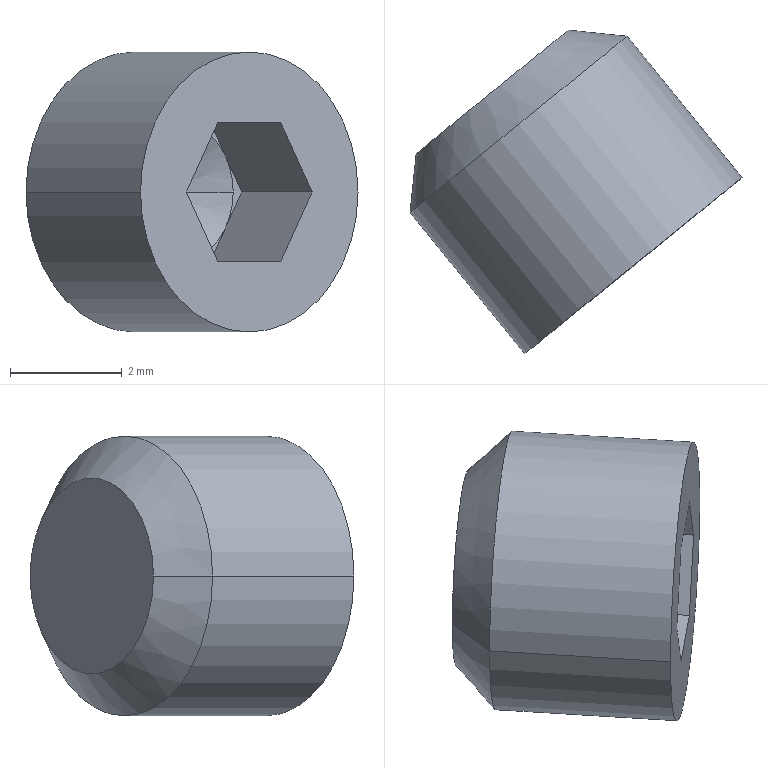Part | SolidWorks | features BaseBody 1 | 1 solid | 20 faces | box 5.931 x 5.783 x 5 mm | volume 62.558 mm3 | plane 14 | cone 4 | cylinder 2 | commonest cylinder face diameters 5 x2
STEP:
#1=CARTESIAN_POINT('',(-125.113,1721.989,-1202.43));
#2=VERTEX_POINT('',#1);
#3=CARTESIAN_POINT('',(-128.998,1718.841,-1202.43));
#4=VERTEX_POINT('',#3);
#5=CARTESIAN_POINT('',(-127.056,1720.415,-1202.43));
#6=DIRECTION('',(0.6296,-0.7769,0.));
#7=DIRECTION('',(0.7769,0.6296,0.));
#8=AXIS2_PLACEMENT_3D('',#5,#6,#7);
#9=CIRCLE('',#8,2.5);
#10=EDGE_CURVE('',#2,#4,#9,.T.);
#11=ORIENTED_EDGE('',*,*,#10,.T.);
#12=CARTESIAN_POINT('',(-126.952,1716.316,-1202.43));
#13=VERTEX_POINT('',#12);
#14=CARTESIAN_POINT('',(-126.952,1716.316,-1202.43));
#15=DIRECTION('',(0.6296,-0.7769,0.));
#16=VECTOR('',#15,1000.);
#17=LINE('',#14,#16);
#18=EDGE_CURVE('',#4,#13,#17,.T.);
#19=ORIENTED_EDGE('',*,*,#18,.T.);
#20=CARTESIAN_POINT('',(-123.067,1719.464,-1202.43));
#21=VERTEX_POINT('',#20);
#22=CARTESIAN_POINT('',(-125.01,1717.89,-1202.43));
#23=DIRECTION('',(-0.6296,0.7769,0.));
#24=DIRECTION('',(0.7769,0.6296,0.));
#25=AXIS2_PLACEMENT_3D('',#22,#23,#24);
#26=CIRCLE('',#25,2.5);
#27=EDGE_CURVE('',#13,#21,#26,.T.);
#28=ORIENTED_EDGE('',*,*,#27,.T.);
#29=CARTESIAN_POINT('',(-123.067,1719.464,-1202.43));
#30=DIRECTION('',(0.6296,-0.7769,0.));
#31=VECTOR('',#30,1000.);
#32=LINE('',#29,#31);
#33=EDGE_CURVE('',#2,#21,#32,.T.);
#34=ORIENTED_EDGE('',*,*,#33,.F.);
#35=EDGE_LOOP('',(#11,#19,#28,#34));
#36=FACE_OUTER_BOUND('',#35,.T.);
#37=CARTESIAN_POINT('',(-125.01,1717.89,-1202.43));
#38=DIRECTION('',(0.6296,-0.7769,0.));
#39=DIRECTION('',(0.7769,0.6296,0.));
#40=AXIS2_PLACEMENT_3D('',#37,#38,#39);
#41=CYLINDRICAL_SURFACE('',#40,2.5);
#42=ADVANCED_FACE('',(#36),#41,.T.);
#43=CARTESIAN_POINT('',(-126.168,1722.1,-1202.43));
#44=VERTEX_POINT('',#43);
#45=CARTESIAN_POINT('',(-128.888,1719.896,-1202.43));
#46=VERTEX_POINT('',#45);
#47=CARTESIAN_POINT('',(-127.528,1720.998,-1202.43));
#48=DIRECTION('',(0.6296,-0.7769,0.));
#49=DIRECTION('',(0.7769,0.6296,0.));
#50=AXIS2_PLACEMENT_3D('',#47,#48,#49);
#51=CIRCLE('',#50,1.75);
#52=EDGE_CURVE('',#44,#46,#51,.T.);
#53=ORIENTED_EDGE('',*,*,#52,.T.);
#54=CARTESIAN_POINT('',(-128.998,1718.841,-1202.43));
#55=DIRECTION('',(-0.1042,-0.9946,0.));
#56=VECTOR('',#55,1000.);
#57=LINE('',#54,#56);
#58=EDGE_CURVE('',#46,#4,#57,.T.);
#59=ORIENTED_EDGE('',*,*,#58,.T.);
#60=ORIENTED_EDGE('',*,*,#10,.F.);
#61=CARTESIAN_POINT('',(-125.113,1721.989,-1202.43));
#62=DIRECTION('',(0.9946,-0.1042,0.));
#63=VECTOR('',#62,1000.);
#64=LINE('',#61,#63);
#65=EDGE_CURVE('',#44,#2,#64,.T.);
#66=ORIENTED_EDGE('',*,*,#65,.F.);
#67=EDGE_LOOP('',(#53,#59,#60,#66));
#68=FACE_OUTER_BOUND('',#67,.T.);
#69=CARTESIAN_POINT('',(-127.056,1720.415,-1202.43));
#70=DIRECTION('',(0.6296,-0.7769,0.));
#71=DIRECTION('',(0.7769,0.6296,0.));
#72=AXIS2_PLACEMENT_3D('',#69,#70,#71);
#73=CONICAL_SURFACE('',#72,2.5,0.7854);
#74=ADVANCED_FACE('',(#68),#73,.T.);
#75=CARTESIAN_POINT('',(-126.723,1720.005,-1202.43));
#76=VERTEX_POINT('',#75);
#77=CARTESIAN_POINT('',(-125.298,1720.231,-1202.43));
#78=VERTEX_POINT('',#77);
#79=CARTESIAN_POINT('',(-125.298,1720.231,-1202.43));
#80=DIRECTION('',(0.9876,0.1568,0.));
#81=VECTOR('',#80,1000.);
#82=LINE('',#79,#81);
#83=EDGE_CURVE('',#76,#78,#82,.T.);
#84=ORIENTED_EDGE('',*,*,#83,.F.);
#85=CARTESIAN_POINT('',(-127.24,1718.657,-1202.43));
#86=VERTEX_POINT('',#85);
#87=CARTESIAN_POINT('',(-127.24,1718.657,-1202.43));
#88=DIRECTION('',(-0.358,-0.9337,0.));
#89=VECTOR('',#88,1000.);
#90=LINE('',#87,#89);
#91=EDGE_CURVE('',#76,#86,#90,.T.);
#92=ORIENTED_EDGE('',*,*,#91,.T.);
#93=CARTESIAN_POINT('',(-127.11,1718.762,-1203.055));
#94=VERTEX_POINT('',#93);
#95=CARTESIAN_POINT('',(-126.269,1719.444,-1202.43));
#96=DIRECTION('',(-0.6296,0.7769,0.));
#97=DIRECTION('',(0.7769,0.6296,0.));
#98=AXIS2_PLACEMENT_3D('',#95,#96,#97);
#99=CIRCLE('',#98,1.25);
#100=EDGE_CURVE('',#94,#86,#99,.T.);
#101=ORIENTED_EDGE('',*,*,#100,.F.);
#102=CARTESIAN_POINT('',(-126.269,1719.444,-1203.68));
#103=VERTEX_POINT('',#102);
#104=CARTESIAN_POINT('',(-126.269,1719.444,-1202.43));
#105=DIRECTION('',(-0.6296,0.7769,0.));
#106=DIRECTION('',(0.7769,0.6296,0.));
#107=AXIS2_PLACEMENT_3D('',#104,#105,#106);
#108=CIRCLE('',#107,1.25);
#109=EDGE_CURVE('',#103,#94,#108,.T.);
#110=ORIENTED_EDGE('',*,*,#109,.F.);
#111=CARTESIAN_POINT('',(-125.428,1720.126,-1203.055));
#112=VERTEX_POINT('',#111);
#113=CARTESIAN_POINT('',(-126.269,1719.444,-1202.43));
#114=DIRECTION('',(-0.6296,0.7769,0.));
#115=DIRECTION('',(0.7769,0.6296,0.));
#116=AXIS2_PLACEMENT_3D('',#113,#114,#115);
#117=CIRCLE('',#116,1.25);
#118=EDGE_CURVE('',#112,#103,#117,.T.);
#119=ORIENTED_EDGE('',*,*,#118,.F.);
#120=CARTESIAN_POINT('',(-126.269,1719.444,-1202.43));
#121=DIRECTION('',(-0.6296,0.7769,0.));
#122=DIRECTION('',(0.7769,0.6296,0.));
#123=AXIS2_PLACEMENT_3D('',#120,#121,#122);
#124=CIRCLE('',#123,1.25);
#125=EDGE_CURVE('',#78,#112,#124,.T.);
#126=ORIENTED_EDGE('',*,*,#125,.F.);
#127=EDGE_LOOP('',(#84,#92,#101,#110,#119,#126));
#128=FACE_OUTER_BOUND('',#127,.T.);
#129=CARTESIAN_POINT('',(-126.269,1719.444,-1202.43));
#130=DIRECTION('',(0.6296,-0.7769,0.));
#131=DIRECTION('',(0.7769,0.6296,0.));
#132=AXIS2_PLACEMENT_3D('',#129,#130,#131);
#133=CONICAL_SURFACE('',#132,1.25,1.047);
#134=ADVANCED_FACE('',(#128),#133,.F.);
#135=ORIENTED_EDGE('',*,*,#18,.F.);
#136=CARTESIAN_POINT('',(-127.056,1720.415,-1202.43));
#137=DIRECTION('',(0.6296,-0.7769,0.));
#138=DIRECTION('',(0.7769,0.6296,0.));
#139=AXIS2_PLACEMENT_3D('',#136,#137,#138);
#140=CIRCLE('',#139,2.5);
#141=EDGE_CURVE('',#4,#2,#140,.T.);
#142=ORIENTED_EDGE('',*,*,#141,.T.);
#143=ORIENTED_EDGE('',*,*,#33,.T.);
#144=CARTESIAN_POINT('',(-125.01,1717.89,-1202.43));
#145=DIRECTION('',(-0.6296,0.7769,0.));
#146=DIRECTION('',(0.7769,0.6296,0.));
#147=AXIS2_PLACEMENT_3D('',#144,#145,#146);
#148=CIRCLE('',#147,2.5);
#149=EDGE_CURVE('',#21,#13,#148,.T.);
#150=ORIENTED_EDGE('',*,*,#149,.T.);
#151=EDGE_LOOP('',(#135,#142,#143,#150));
#152=FACE_OUTER_BOUND('',#151,.T.);
#153=CARTESIAN_POINT('',(-125.01,1717.89,-1202.43));
#154=DIRECTION('',(0.6296,-0.7769,0.));
#155=DIRECTION('',(0.7769,0.6296,0.));
#156=AXIS2_PLACEMENT_3D('',#153,#154,#155);
#157=CYLINDRICAL_SURFACE('',#156,2.5);
#158=ADVANCED_FACE('',(#152),#157,.T.);
#159=CARTESIAN_POINT('',(-125.57,1717.436,-1203.68));
#160=VERTEX_POINT('',#159);
#161=CARTESIAN_POINT('',(-124.449,1718.344,-1203.68));
#162=VERTEX_POINT('',#161);
#163=CARTESIAN_POINT('',(-125.01,1717.89,-1203.68));
#164=DIRECTION('',(0.7769,0.6296,0.));
#165=VECTOR('',#164,1000.);
#166=LINE('',#163,#165);
#167=EDGE_CURVE('',#160,#162,#166,.T.);
#168=ORIENTED_EDGE('',*,*,#167,.F.);
#169=CARTESIAN_POINT('',(-126.131,1716.981,-1202.43));
#170=VERTEX_POINT('',#169);
#171=CARTESIAN_POINT('',(-126.131,1716.981,-1202.43));
#172=DIRECTION('',(0.3885,0.3148,-0.866));
#173=VECTOR('',#172,1000.);
#174=LINE('',#171,#173);
#175=EDGE_CURVE('',#170,#160,#174,.T.);
#176=ORIENTED_EDGE('',*,*,#175,.F.);
#177=CARTESIAN_POINT('',(-125.57,1717.436,-1201.18));
#178=VERTEX_POINT('',#177);
#179=CARTESIAN_POINT('',(-125.57,1717.436,-1201.18));
#180=DIRECTION('',(-0.3885,-0.3148,-0.866));
#181=VECTOR('',#180,1000.);
#182=LINE('',#179,#181);
#183=EDGE_CURVE('',#178,#170,#182,.T.);
#184=ORIENTED_EDGE('',*,*,#183,.F.);
#185=CARTESIAN_POINT('',(-124.449,1718.344,-1201.18));
#186=VERTEX_POINT('',#185);
#187=CARTESIAN_POINT('',(-125.01,1717.89,-1201.18));
#188=DIRECTION('',(-0.7769,-0.6296,0.));
#189=VECTOR('',#188,1000.);
#190=LINE('',#187,#189);
#191=EDGE_CURVE('',#186,#178,#190,.T.);
#192=ORIENTED_EDGE('',*,*,#191,.F.);
#193=CARTESIAN_POINT('',(-123.888,1718.799,-1202.43));
#194=VERTEX_POINT('',#193);
#195=CARTESIAN_POINT('',(-123.888,1718.799,-1202.43));
#196=DIRECTION('',(-0.3885,-0.3148,0.866));
#197=VECTOR('',#196,1000.);
#198=LINE('',#195,#197);
#199=EDGE_CURVE('',#194,#186,#198,.T.);
#200=ORIENTED_EDGE('',*,*,#199,.F.);
#201=CARTESIAN_POINT('',(-124.449,1718.344,-1203.68));
#202=DIRECTION('',(0.3885,0.3148,0.866));
#203=VECTOR('',#202,1000.);
#204=LINE('',#201,#203);
#205=EDGE_CURVE('',#162,#194,#204,.T.);
#206=ORIENTED_EDGE('',*,*,#205,.F.);
#207=EDGE_LOOP('',(#168,#176,#184,#192,#200,#206));
#208=FACE_BOUND('',#207,.T.);
#209=ORIENTED_EDGE('',*,*,#149,.F.);
#210=ORIENTED_EDGE('',*,*,#27,.F.);
#211=EDGE_LOOP('',(#209,#210));
#212=FACE_OUTER_BOUND('',#211,.T.);
#213=CARTESIAN_POINT('',(-125.01,1717.89,-1202.43));
#214=DIRECTION('',(-0.6296,0.7769,0.));
#215=DIRECTION('',(-0.7769,-0.6296,0.));
#216=AXIS2_PLACEMENT_3D('',#213,#214,#215);
#217=PLANE('',#216);
#218=ADVANCED_FACE('',(#208,#212),#217,.F.);
#219=ORIENTED_EDGE('',*,*,#58,.F.);
#220=CARTESIAN_POINT('',(-127.528,1720.998,-1202.43));
#221=DIRECTION('',(0.6296,-0.7769,0.));
#222=DIRECTION('',(0.7769,0.6296,0.));
#223=AXIS2_PLACEMENT_3D('',#220,#221,#222);
#224=CIRCLE('',#223,1.75);
#225=EDGE_CURVE('',#46,#44,#224,.T.);
#226=ORIENTED_EDGE('',*,*,#225,.T.);
#227=ORIENTED_EDGE('',*,*,#65,.T.);
#228=ORIENTED_EDGE('',*,*,#141,.F.);
#229=EDGE_LOOP('',(#219,#226,#227,#228));
#230=FACE_OUTER_BOUND('',#229,.T.);
#231=CARTESIAN_POINT('',(-127.056,1720.415,-1202.43));
#232=DIRECTION('',(0.6296,-0.7769,0.));
#233=DIRECTION('',(0.7769,0.6296,0.));
#234=AXIS2_PLACEMENT_3D('',#231,#232,#233);
#235=CONICAL_SURFACE('',#234,2.5,0.7854);
#236=ADVANCED_FACE('',(#230),#235,.T.);
#237=ORIENTED_EDGE('',*,*,#205,.T.);
#238=CARTESIAN_POINT('',(-125.147,1720.353,-1202.43));
#239=VERTEX_POINT('',#238);
#240=CARTESIAN_POINT('',(-125.147,1720.353,-1202.43));
#241=DIRECTION('',(0.6296,-0.7769,0.));
#242=VECTOR('',#241,1000.);
#243=LINE('',#240,#242);
#244=EDGE_CURVE('',#239,#194,#243,.T.);
#245=ORIENTED_EDGE('',*,*,#244,.F.);
#246=CARTESIAN_POINT('',(-125.708,1719.898,-1203.68));
#247=DIRECTION('',(0.3885,0.3148,0.866));
#248=VECTOR('',#247,1000.);
#249=LINE('',#246,#248);
#250=EDGE_CURVE('',#112,#239,#249,.T.);
#251=ORIENTED_EDGE('',*,*,#250,.F.);
#252=CARTESIAN_POINT('',(-125.708,1719.898,-1203.68));
#253=VERTEX_POINT('',#252);
#254=CARTESIAN_POINT('',(-125.708,1719.898,-1203.68));
#255=DIRECTION('',(0.3885,0.3148,0.866));
#256=VECTOR('',#255,1000.);
#257=LINE('',#254,#256);
#258=EDGE_CURVE('',#253,#112,#257,.T.);
#259=ORIENTED_EDGE('',*,*,#258,.F.);
#260=CARTESIAN_POINT('',(-125.708,1719.898,-1203.68));
#261=DIRECTION('',(-0.6296,0.7769,0.));
#262=VECTOR('',#261,1000.);
#263=LINE('',#260,#262);
#264=EDGE_CURVE('',#162,#253,#263,.T.);
#265=ORIENTED_EDGE('',*,*,#264,.F.);
#266=EDGE_LOOP('',(#237,#245,#251,#259,#265));
#267=FACE_OUTER_BOUND('',#266,.T.);
#268=CARTESIAN_POINT('',(-125.708,1719.898,-1203.68));
#269=DIRECTION('',(0.6728,0.5452,-0.5));
#270=DIRECTION('',(-0.6296,0.7769,0.));
#271=AXIS2_PLACEMENT_3D('',#268,#269,#270);
#272=PLANE('',#271);
#273=ADVANCED_FACE('',(#267),#272,.F.);
#274=ORIENTED_EDGE('',*,*,#167,.T.);
#275=ORIENTED_EDGE('',*,*,#264,.T.);
#276=CARTESIAN_POINT('',(-126.269,1719.444,-1203.68));
#277=DIRECTION('',(0.7769,0.6296,0.));
#278=VECTOR('',#277,1000.);
#279=LINE('',#276,#278);
#280=EDGE_CURVE('',#103,#253,#279,.T.);
#281=ORIENTED_EDGE('',*,*,#280,.F.);
#282=CARTESIAN_POINT('',(-126.829,1718.99,-1203.68));
#283=VERTEX_POINT('',#282);
#284=CARTESIAN_POINT('',(-126.829,1718.99,-1203.68));
#285=DIRECTION('',(0.7769,0.6296,0.));
#286=VECTOR('',#285,1000.);
#287=LINE('',#284,#286);
#288=EDGE_CURVE('',#283,#103,#287,.T.);
#289=ORIENTED_EDGE('',*,*,#288,.F.);
#290=CARTESIAN_POINT('',(-125.57,1717.436,-1203.68));
#291=DIRECTION('',(-0.6296,0.7769,0.));
#292=VECTOR('',#291,1000.);
#293=LINE('',#290,#292);
#294=EDGE_CURVE('',#160,#283,#293,.T.);
#295=ORIENTED_EDGE('',*,*,#294,.F.);
#296=EDGE_LOOP('',(#274,#275,#281,#289,#295));
#297=FACE_OUTER_BOUND('',#296,.T.);
#298=CARTESIAN_POINT('',(-126.829,1718.99,-1203.68));
#299=DIRECTION('',(0.,0.,-1.));
#300=DIRECTION('',(-1.,0.,0.));
#301=AXIS2_PLACEMENT_3D('',#298,#299,#300);
#302=PLANE('',#301);
#303=ADVANCED_FACE('',(#297),#302,.F.);
#304=ORIENTED_EDGE('',*,*,#175,.T.);
#305=ORIENTED_EDGE('',*,*,#294,.T.);
#306=CARTESIAN_POINT('',(-127.39,1718.535,-1202.43));
#307=DIRECTION('',(0.3885,0.3148,-0.866));
#308=VECTOR('',#307,1000.);
#309=LINE('',#306,#308);
#310=EDGE_CURVE('',#94,#283,#309,.T.);
#311=ORIENTED_EDGE('',*,*,#310,.F.);
#312=CARTESIAN_POINT('',(-127.39,1718.535,-1202.43));
#313=VERTEX_POINT('',#312);
#314=CARTESIAN_POINT('',(-127.39,1718.535,-1202.43));
#315=DIRECTION('',(0.3885,0.3148,-0.866));
#316=VECTOR('',#315,1000.);
#317=LINE('',#314,#316);
#318=EDGE_CURVE('',#313,#94,#317,.T.);
#319=ORIENTED_EDGE('',*,*,#318,.F.);
#320=CARTESIAN_POINT('',(-127.39,1718.535,-1202.43));
#321=DIRECTION('',(-0.6296,0.7769,0.));
#322=VECTOR('',#321,1000.);
#323=LINE('',#320,#322);
#324=EDGE_CURVE('',#170,#313,#323,.T.);
#325=ORIENTED_EDGE('',*,*,#324,.F.);
#326=EDGE_LOOP('',(#304,#305,#311,#319,#325));
#327=FACE_OUTER_BOUND('',#326,.T.);
#328=CARTESIAN_POINT('',(-127.39,1718.535,-1202.43));
#329=DIRECTION('',(-0.6728,-0.5452,-0.5));
#330=DIRECTION('',(0.6296,-0.7769,0.));
#331=AXIS2_PLACEMENT_3D('',#328,#329,#330);
#332=PLANE('',#331);
#333=ADVANCED_FACE('',(#327),#332,.F.);
#334=ORIENTED_EDGE('',*,*,#183,.T.);
#335=ORIENTED_EDGE('',*,*,#324,.T.);
#336=CARTESIAN_POINT('',(-127.11,1718.762,-1201.805));
#337=VERTEX_POINT('',#336);
#338=CARTESIAN_POINT('',(-126.829,1718.99,-1201.18));
#339=DIRECTION('',(-0.3885,-0.3148,-0.866));
#340=VECTOR('',#339,1000.);
#341=LINE('',#338,#340);
#342=EDGE_CURVE('',#337,#313,#341,.T.);
#343=ORIENTED_EDGE('',*,*,#342,.F.);
#344=CARTESIAN_POINT('',(-126.829,1718.99,-1201.18));
#345=VERTEX_POINT('',#344);
#346=CARTESIAN_POINT('',(-126.829,1718.99,-1201.18));
#347=DIRECTION('',(-0.3885,-0.3148,-0.866));
#348=VECTOR('',#347,1000.);
#349=LINE('',#346,#348);
#350=EDGE_CURVE('',#345,#337,#349,.T.);
#351=ORIENTED_EDGE('',*,*,#350,.F.);
#352=CARTESIAN_POINT('',(-126.829,1718.99,-1201.18));
#353=DIRECTION('',(-0.6296,0.7769,0.));
#354=VECTOR('',#353,1000.);
#355=LINE('',#352,#354);
#356=EDGE_CURVE('',#178,#345,#355,.T.);
#357=ORIENTED_EDGE('',*,*,#356,.F.);
#358=EDGE_LOOP('',(#334,#335,#343,#351,#357));
#359=FACE_OUTER_BOUND('',#358,.T.);
#360=CARTESIAN_POINT('',(-126.829,1718.99,-1201.18));
#361=DIRECTION('',(-0.6728,-0.5452,0.5));
#362=DIRECTION('',(0.6296,-0.7769,0.));
#363=AXIS2_PLACEMENT_3D('',#360,#361,#362);
#364=PLANE('',#363);
#365=ADVANCED_FACE('',(#359),#364,.F.);
#366=ORIENTED_EDGE('',*,*,#191,.T.);
#367=ORIENTED_EDGE('',*,*,#356,.T.);
#368=CARTESIAN_POINT('',(-126.269,1719.444,-1201.18));
#369=VERTEX_POINT('',#368);
#370=CARTESIAN_POINT('',(-126.269,1719.444,-1201.18));
#371=DIRECTION('',(-0.7769,-0.6296,0.));
#372=VECTOR('',#371,1000.);
#373=LINE('',#370,#372);
#374=EDGE_CURVE('',#369,#345,#373,.T.);
#375=ORIENTED_EDGE('',*,*,#374,.F.);
#376=CARTESIAN_POINT('',(-125.708,1719.898,-1201.18));
#377=VERTEX_POINT('',#376);
#378=CARTESIAN_POINT('',(-125.708,1719.898,-1201.18));
#379=DIRECTION('',(-0.7769,-0.6296,0.));
#380=VECTOR('',#379,1000.);
#381=LINE('',#378,#380);
#382=EDGE_CURVE('',#377,#369,#381,.T.);
#383=ORIENTED_EDGE('',*,*,#382,.F.);
#384=CARTESIAN_POINT('',(-124.449,1718.344,-1201.18));
#385=DIRECTION('',(-0.6296,0.7769,0.));
#386=VECTOR('',#385,1000.);
#387=LINE('',#384,#386);
#388=EDGE_CURVE('',#186,#377,#387,.T.);
#389=ORIENTED_EDGE('',*,*,#388,.F.);
#390=EDGE_LOOP('',(#366,#367,#375,#383,#389));
#391=FACE_OUTER_BOUND('',#390,.T.);
#392=CARTESIAN_POINT('',(-125.708,1719.898,-1201.18));
#393=DIRECTION('',(0.,0.,1.));
#394=DIRECTION('',(1.,0.,0.));
#395=AXIS2_PLACEMENT_3D('',#392,#393,#394);
#396=PLANE('',#395);
#397=ADVANCED_FACE('',(#391),#396,.F.);
#398=ORIENTED_EDGE('',*,*,#199,.T.);
#399=ORIENTED_EDGE('',*,*,#388,.T.);
#400=CARTESIAN_POINT('',(-125.428,1720.126,-1201.805));
#401=VERTEX_POINT('',#400);
#402=CARTESIAN_POINT('',(-125.147,1720.353,-1202.43));
#403=DIRECTION('',(-0.3885,-0.3148,0.866));
#404=VECTOR('',#403,1000.);
#405=LINE('',#402,#404);
#406=EDGE_CURVE('',#401,#377,#405,.T.);
#407=ORIENTED_EDGE('',*,*,#406,.F.);
#408=CARTESIAN_POINT('',(-125.147,1720.353,-1202.43));
#409=DIRECTION('',(-0.3885,-0.3148,0.866));
#410=VECTOR('',#409,1000.);
#411=LINE('',#408,#410);
#412=EDGE_CURVE('',#239,#401,#411,.T.);
#413=ORIENTED_EDGE('',*,*,#412,.F.);
#414=ORIENTED_EDGE('',*,*,#244,.T.);
#415=EDGE_LOOP('',(#398,#399,#407,#413,#414));
#416=FACE_OUTER_BOUND('',#415,.T.);
#417=CARTESIAN_POINT('',(-125.147,1720.353,-1202.43));
#418=DIRECTION('',(0.6728,0.5452,0.5));
#419=DIRECTION('',(-0.6296,0.7769,0.));
#420=AXIS2_PLACEMENT_3D('',#417,#418,#419);
#421=PLANE('',#420);
#422=ADVANCED_FACE('',(#416),#421,.F.);
#423=ORIENTED_EDGE('',*,*,#52,.F.);
#424=ORIENTED_EDGE('',*,*,#225,.F.);
#425=EDGE_LOOP('',(#423,#424));
#426=FACE_OUTER_BOUND('',#425,.T.);
#427=CARTESIAN_POINT('',(-127.528,1720.998,-1202.43));
#428=DIRECTION('',(0.6296,-0.7769,0.));
#429=DIRECTION('',(0.7769,0.6296,0.));
#430=AXIS2_PLACEMENT_3D('',#427,#428,#429);
#431=PLANE('',#430);
#432=ADVANCED_FACE('',(#426),#431,.F.);
#433=CARTESIAN_POINT('',(-126.269,1719.444,-1202.43));
#434=DIRECTION('',(-0.6296,0.7769,0.));
#435=DIRECTION('',(0.7769,0.6296,0.));
#436=AXIS2_PLACEMENT_3D('',#433,#434,#435);
#437=CIRCLE('',#436,1.25);
#438=EDGE_CURVE('',#401,#78,#437,.T.);
#439=ORIENTED_EDGE('',*,*,#438,.T.);
#440=ORIENTED_EDGE('',*,*,#125,.T.);
#441=ORIENTED_EDGE('',*,*,#250,.T.);
#442=ORIENTED_EDGE('',*,*,#412,.T.);
#443=EDGE_LOOP('',(#439,#440,#441,#442));
#444=FACE_OUTER_BOUND('',#443,.T.);
#445=CARTESIAN_POINT('',(-126.269,1719.444,-1202.43));
#446=DIRECTION('',(0.6296,-0.7769,0.));
#447=DIRECTION('',(0.7769,0.6296,0.));
#448=AXIS2_PLACEMENT_3D('',#445,#446,#447);
#449=PLANE('',#448);
#450=ADVANCED_FACE('',(#444),#449,.T.);
#451=ORIENTED_EDGE('',*,*,#118,.T.);
#452=ORIENTED_EDGE('',*,*,#280,.T.);
#453=ORIENTED_EDGE('',*,*,#258,.T.);
#454=EDGE_LOOP('',(#451,#452,#453));
#455=FACE_OUTER_BOUND('',#454,.T.);
#456=CARTESIAN_POINT('',(-126.269,1719.444,-1202.43));
#457=DIRECTION('',(0.6296,-0.7769,0.));
#458=DIRECTION('',(0.7769,0.6296,0.));
#459=AXIS2_PLACEMENT_3D('',#456,#457,#458);
#460=PLANE('',#459);
#461=ADVANCED_FACE('',(#455),#460,.T.);
#462=ORIENTED_EDGE('',*,*,#109,.T.);
#463=ORIENTED_EDGE('',*,*,#310,.T.);
#464=ORIENTED_EDGE('',*,*,#288,.T.);
#465=EDGE_LOOP('',(#462,#463,#464));
#466=FACE_OUTER_BOUND('',#465,.T.);
#467=CARTESIAN_POINT('',(-126.269,1719.444,-1202.43));
#468=DIRECTION('',(0.6296,-0.7769,0.));
#469=DIRECTION('',(0.7769,0.6296,0.));
#470=AXIS2_PLACEMENT_3D('',#467,#468,#469);
#471=PLANE('',#470);
#472=ADVANCED_FACE('',(#466),#471,.T.);
#473=ORIENTED_EDGE('',*,*,#100,.T.);
#474=CARTESIAN_POINT('',(-126.269,1719.444,-1202.43));
#475=DIRECTION('',(-0.6296,0.7769,0.));
#476=DIRECTION('',(0.7769,0.6296,0.));
#477=AXIS2_PLACEMENT_3D('',#474,#475,#476);
#478=CIRCLE('',#477,1.25);
#479=EDGE_CURVE('',#86,#337,#478,.T.);
#480=ORIENTED_EDGE('',*,*,#479,.T.);
#481=ORIENTED_EDGE('',*,*,#342,.T.);
#482=ORIENTED_EDGE('',*,*,#318,.T.);
#483=EDGE_LOOP('',(#473,#480,#481,#482));
#484=FACE_OUTER_BOUND('',#483,.T.);
#485=CARTESIAN_POINT('',(-126.269,1719.444,-1202.43));
#486=DIRECTION('',(0.6296,-0.7769,0.));
#487=DIRECTION('',(0.7769,0.6296,0.));
#488=AXIS2_PLACEMENT_3D('',#485,#486,#487);
#489=PLANE('',#488);
#490=ADVANCED_FACE('',(#484),#489,.T.);
#491=CARTESIAN_POINT('',(-126.269,1719.444,-1202.43));
#492=DIRECTION('',(-0.6296,0.7769,0.));
#493=DIRECTION('',(0.7769,0.6296,0.));
#494=AXIS2_PLACEMENT_3D('',#491,#492,#493);
#495=CIRCLE('',#494,1.25);
#496=EDGE_CURVE('',#337,#369,#495,.T.);
#497=ORIENTED_EDGE('',*,*,#496,.T.);
#498=ORIENTED_EDGE('',*,*,#374,.T.);
#499=ORIENTED_EDGE('',*,*,#350,.T.);
#500=EDGE_LOOP('',(#497,#498,#499));
#501=FACE_OUTER_BOUND('',#500,.T.);
#502=CARTESIAN_POINT('',(-126.269,1719.444,-1202.43));
#503=DIRECTION('',(0.6296,-0.7769,0.));
#504=DIRECTION('',(0.7769,0.6296,0.));
#505=AXIS2_PLACEMENT_3D('',#502,#503,#504);
#506=PLANE('',#505);
#507=ADVANCED_FACE('',(#501),#506,.T.);
#508=CARTESIAN_POINT('',(-126.269,1719.444,-1202.43));
#509=DIRECTION('',(-0.6296,0.7769,0.));
#510=DIRECTION('',(0.7769,0.6296,0.));
#511=AXIS2_PLACEMENT_3D('',#508,#509,#510);
#512=CIRCLE('',#511,1.25);
#513=EDGE_CURVE('',#369,#401,#512,.T.);
#514=ORIENTED_EDGE('',*,*,#513,.T.);
#515=ORIENTED_EDGE('',*,*,#406,.T.);
#516=ORIENTED_EDGE('',*,*,#382,.T.);
#517=EDGE_LOOP('',(#514,#515,#516));
#518=FACE_OUTER_BOUND('',#517,.T.);
#519=CARTESIAN_POINT('',(-126.269,1719.444,-1202.43));
#520=DIRECTION('',(0.6296,-0.7769,0.));
#521=DIRECTION('',(0.7769,0.6296,0.));
#522=AXIS2_PLACEMENT_3D('',#519,#520,#521);
#523=PLANE('',#522);
#524=ADVANCED_FACE('',(#518),#523,.T.);
#525=ORIENTED_EDGE('',*,*,#91,.F.);
#526=ORIENTED_EDGE('',*,*,#83,.T.);
#527=ORIENTED_EDGE('',*,*,#438,.F.);
#528=ORIENTED_EDGE('',*,*,#513,.F.);
#529=ORIENTED_EDGE('',*,*,#496,.F.);
#530=ORIENTED_EDGE('',*,*,#479,.F.);
#531=EDGE_LOOP('',(#525,#526,#527,#528,#529,#530));
#532=FACE_OUTER_BOUND('',#531,.T.);
#533=CARTESIAN_POINT('',(-126.269,1719.444,-1202.43));
#534=DIRECTION('',(0.6296,-0.7769,0.));
#535=DIRECTION('',(0.7769,0.6296,0.));
#536=AXIS2_PLACEMENT_3D('',#533,#534,#535);
#537=CONICAL_SURFACE('',#536,1.25,1.047);
#538=ADVANCED_FACE('',(#532),#537,.F.);
#539=CLOSED_SHELL('',(#42,#74,#134,#158,#218,#236,#273,#303,#333,#365,#397,#422,#432,#450,#461,#472,#490,#507,#524,#538));
#540=MANIFOLD_SOLID_BREP('',#539);
#541=CARTESIAN_POINT('',(0.,0.,0.));
#542=DIRECTION('',(0.,0.,1.));
#543=DIRECTION('',(1.,0.,0.));
#544=AXIS2_PLACEMENT_3D('',#541,#542,#543);
#545=(LENGTH_UNIT()NAMED_UNIT(*)SI_UNIT(.MILLI.,.METRE.));
#546=UNCERTAINTY_MEASURE_WITH_UNIT(LENGTH_MEASURE(0.00001),#545,'','');
#547=(NAMED_UNIT(*)PLANE_ANGLE_UNIT()SI_UNIT($,.RADIAN.));
#548=(NAMED_UNIT(*)SI_UNIT($,.STERADIAN.)SOLID_ANGLE_UNIT());
#549=(GEOMETRIC_REPRESENTATION_CONTEXT(3)GLOBAL_UNCERTAINTY_ASSIGNED_CONTEXT((#546))GLOBAL_UNIT_ASSIGNED_CONTEXT((#545,#547,#548))REPRESENTATION_CONTEXT('',''));
#550=ADVANCED_BREP_SHAPE_REPRESENTATION('',(#540,#544),#549);